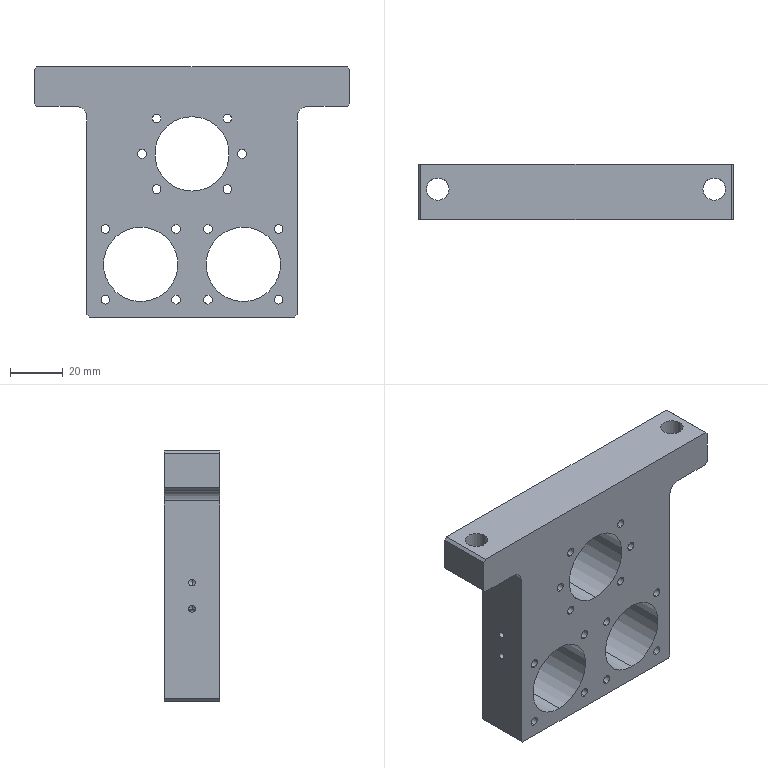Part | STEP file | Left Moving Support Plate | 1 solid | 72 faces | box 120 x 21 x 95 mm | volume 128293 mm3 | cylinder 48 | plane 16 | cone 8 | commonest cylinder face diameters 3.3 x28 2.5 x8 28.3 x6 8.5 x4 8 x2